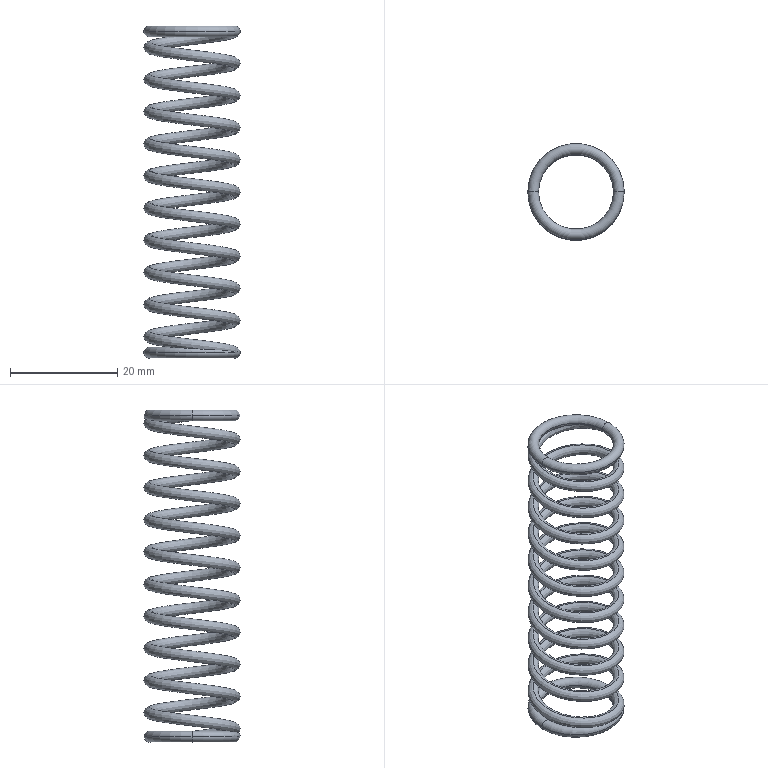Part | NX | features BREP 1 | 1 solid | 10 faces | box 18 x 18 x 62 mm | volume 1869 mm3 | torus 8 | spline 2